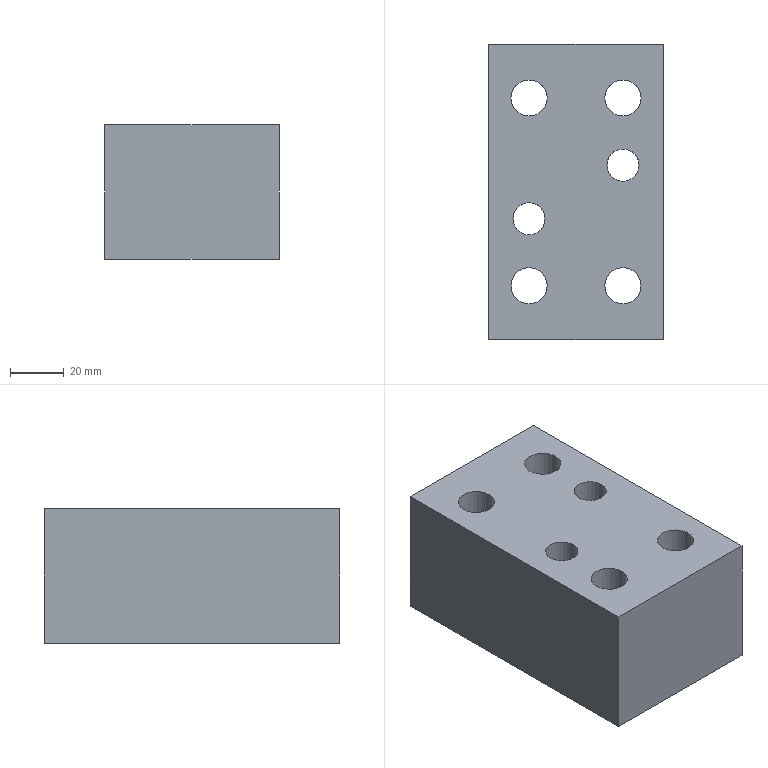Part | NX | features solid 2 | 1 solid | 20 faces | box 65 x 110 x 50 mm | volume 298901 mm3 | plane 10 | cylinder 10 | commonest cylinder face diameters 13.5 x4 19.5 x4 12 x2
STEP:
#1=CARTESIAN_POINT('',(-997.,18.,20.));
#2=VERTEX_POINT('',#1);
#3=CARTESIAN_POINT('',(-1003.,18.,20.));
#4=DIRECTION('',(0.,0.,1.));
#5=DIRECTION('',(1.,0.,0.));
#6=AXIS2_PLACEMENT_3D('',#3,#4,#5);
#7=CIRCLE('',#6,6.);
#8=EDGE_CURVE('',#2,#2,#7,.F.);
#9=ORIENTED_EDGE('',*,*,#8,.F.);
#10=EDGE_LOOP('',(#9));
#11=FACE_BOUND('',#10,.T.);
#12=CARTESIAN_POINT('',(-993.25,43.,20.));
#13=VERTEX_POINT('',#12);
#14=CARTESIAN_POINT('',(-1003.,43.,20.));
#15=DIRECTION('',(0.,0.,1.));
#16=DIRECTION('',(1.,0.,0.));
#17=AXIS2_PLACEMENT_3D('',#14,#15,#16);
#18=CIRCLE('',#17,9.75);
#19=EDGE_CURVE('',#13,#13,#18,.F.);
#20=ORIENTED_EDGE('',*,*,#19,.F.);
#21=EDGE_LOOP('',(#20));
#22=FACE_BOUND('',#21,.T.);
#23=CARTESIAN_POINT('',(-1028.25,-27.,20.));
#24=VERTEX_POINT('',#23);
#25=CARTESIAN_POINT('',(-1038.,-27.,20.));
#26=DIRECTION('',(0.,0.,1.));
#27=DIRECTION('',(1.,0.,0.));
#28=AXIS2_PLACEMENT_3D('',#25,#26,#27);
#29=CIRCLE('',#28,9.75);
#30=EDGE_CURVE('',#24,#24,#29,.F.);
#31=ORIENTED_EDGE('',*,*,#30,.F.);
#32=EDGE_LOOP('',(#31));
#33=FACE_BOUND('',#32,.T.);
#34=CARTESIAN_POINT('',(-1053.,63.,20.));
#35=VERTEX_POINT('',#34);
#36=CARTESIAN_POINT('',(-988.,63.,20.));
#37=VERTEX_POINT('',#36);
#38=CARTESIAN_POINT('',(-1028.,63.,20.));
#39=DIRECTION('',(1.,0.,0.));
#40=VECTOR('',#39,1000.);
#41=LINE('',#38,#40);
#42=EDGE_CURVE('',#35,#37,#41,.T.);
#43=ORIENTED_EDGE('',*,*,#42,.T.);
#44=CARTESIAN_POINT('',(-988.,-47.,20.));
#45=VERTEX_POINT('',#44);
#46=CARTESIAN_POINT('',(-988.,8.,20.));
#47=DIRECTION('',(0.,-1.,0.));
#48=VECTOR('',#47,1000.);
#49=LINE('',#46,#48);
#50=EDGE_CURVE('',#37,#45,#49,.T.);
#51=ORIENTED_EDGE('',*,*,#50,.T.);
#52=CARTESIAN_POINT('',(-1053.,-47.,20.));
#53=VERTEX_POINT('',#52);
#54=CARTESIAN_POINT('',(-1028.,-47.,20.));
#55=DIRECTION('',(1.,0.,0.));
#56=VECTOR('',#55,1000.);
#57=LINE('',#54,#56);
#58=EDGE_CURVE('',#53,#45,#57,.T.);
#59=ORIENTED_EDGE('',*,*,#58,.F.);
#60=CARTESIAN_POINT('',(-1053.,8.,20.));
#61=DIRECTION('',(0.,-1.,0.));
#62=VECTOR('',#61,1000.);
#63=LINE('',#60,#62);
#64=EDGE_CURVE('',#35,#53,#63,.T.);
#65=ORIENTED_EDGE('',*,*,#64,.F.);
#66=EDGE_LOOP('',(#43,#51,#59,#65));
#67=FACE_BOUND('',#66,.T.);
#68=CARTESIAN_POINT('',(-1028.25,43.,20.));
#69=VERTEX_POINT('',#68);
#70=CARTESIAN_POINT('',(-1038.,43.,20.));
#71=DIRECTION('',(0.,0.,1.));
#72=DIRECTION('',(1.,0.,0.));
#73=AXIS2_PLACEMENT_3D('',#70,#71,#72);
#74=CIRCLE('',#73,9.75);
#75=EDGE_CURVE('',#69,#69,#74,.F.);
#76=ORIENTED_EDGE('',*,*,#75,.F.);
#77=EDGE_LOOP('',(#76));
#78=FACE_BOUND('',#77,.T.);
#79=CARTESIAN_POINT('',(-993.25,-27.,20.));
#80=VERTEX_POINT('',#79);
#81=CARTESIAN_POINT('',(-1003.,-27.,20.));
#82=DIRECTION('',(0.,0.,1.));
#83=DIRECTION('',(1.,0.,0.));
#84=AXIS2_PLACEMENT_3D('',#81,#82,#83);
#85=CIRCLE('',#84,9.75);
#86=EDGE_CURVE('',#80,#80,#85,.F.);
#87=ORIENTED_EDGE('',*,*,#86,.F.);
#88=EDGE_LOOP('',(#87));
#89=FACE_BOUND('',#88,.T.);
#90=CARTESIAN_POINT('',(-1032.,-2.,20.));
#91=VERTEX_POINT('',#90);
#92=CARTESIAN_POINT('',(-1038.,-2.,20.));
#93=DIRECTION('',(0.,0.,1.));
#94=DIRECTION('',(1.,0.,0.));
#95=AXIS2_PLACEMENT_3D('',#92,#93,#94);
#96=CIRCLE('',#95,6.);
#97=EDGE_CURVE('',#91,#91,#96,.F.);
#98=ORIENTED_EDGE('',*,*,#97,.F.);
#99=EDGE_LOOP('',(#98));
#100=FACE_BOUND('',#99,.T.);
#101=CARTESIAN_POINT('',(-1028.,8.,20.));
#102=DIRECTION('',(0.,0.,1.));
#103=DIRECTION('',(0.,-1.,0.));
#104=AXIS2_PLACEMENT_3D('',#101,#102,#103);
#105=PLANE('',#104);
#106=ADVANCED_FACE('',(#11,#22,#33,#67,#78,#89,#100),#105,.F.);
#107=CARTESIAN_POINT('',(-997.,18.,70.));
#108=VERTEX_POINT('',#107);
#109=CARTESIAN_POINT('',(-1003.,18.,70.));
#110=DIRECTION('',(0.,0.,1.));
#111=DIRECTION('',(1.,0.,0.));
#112=AXIS2_PLACEMENT_3D('',#109,#110,#111);
#113=CIRCLE('',#112,6.);
#114=EDGE_CURVE('',#108,#108,#113,.F.);
#115=ORIENTED_EDGE('',*,*,#114,.T.);
#116=EDGE_LOOP('',(#115));
#117=FACE_BOUND('',#116,.T.);
#118=CARTESIAN_POINT('',(-1031.25,43.,70.));
#119=VERTEX_POINT('',#118);
#120=CARTESIAN_POINT('',(-1038.,43.,70.));
#121=DIRECTION('',(0.,0.,1.));
#122=DIRECTION('',(1.,0.,0.));
#123=AXIS2_PLACEMENT_3D('',#120,#121,#122);
#124=CIRCLE('',#123,6.75);
#125=EDGE_CURVE('',#119,#119,#124,.T.);
#126=ORIENTED_EDGE('',*,*,#125,.F.);
#127=EDGE_LOOP('',(#126));
#128=FACE_BOUND('',#127,.T.);
#129=CARTESIAN_POINT('',(-996.25,-27.,70.));
#130=VERTEX_POINT('',#129);
#131=CARTESIAN_POINT('',(-1003.,-27.,70.));
#132=DIRECTION('',(0.,0.,1.));
#133=DIRECTION('',(1.,0.,0.));
#134=AXIS2_PLACEMENT_3D('',#131,#132,#133);
#135=CIRCLE('',#134,6.75);
#136=EDGE_CURVE('',#130,#130,#135,.T.);
#137=ORIENTED_EDGE('',*,*,#136,.F.);
#138=EDGE_LOOP('',(#137));
#139=FACE_BOUND('',#138,.T.);
#140=CARTESIAN_POINT('',(-1053.,63.,70.));
#141=VERTEX_POINT('',#140);
#142=CARTESIAN_POINT('',(-988.,63.,70.));
#143=VERTEX_POINT('',#142);
#144=CARTESIAN_POINT('',(-1028.,63.,70.));
#145=DIRECTION('',(1.,0.,0.));
#146=VECTOR('',#145,1000.);
#147=LINE('',#144,#146);
#148=EDGE_CURVE('',#141,#143,#147,.T.);
#149=ORIENTED_EDGE('',*,*,#148,.F.);
#150=CARTESIAN_POINT('',(-1053.,-47.,70.));
#151=VERTEX_POINT('',#150);
#152=CARTESIAN_POINT('',(-1053.,8.,70.));
#153=DIRECTION('',(0.,-1.,0.));
#154=VECTOR('',#153,1000.);
#155=LINE('',#152,#154);
#156=EDGE_CURVE('',#141,#151,#155,.T.);
#157=ORIENTED_EDGE('',*,*,#156,.T.);
#158=CARTESIAN_POINT('',(-988.,-47.,70.));
#159=VERTEX_POINT('',#158);
#160=CARTESIAN_POINT('',(-1028.,-47.,70.));
#161=DIRECTION('',(1.,0.,0.));
#162=VECTOR('',#161,1000.);
#163=LINE('',#160,#162);
#164=EDGE_CURVE('',#151,#159,#163,.T.);
#165=ORIENTED_EDGE('',*,*,#164,.T.);
#166=CARTESIAN_POINT('',(-988.,8.,70.));
#167=DIRECTION('',(0.,-1.,0.));
#168=VECTOR('',#167,1000.);
#169=LINE('',#166,#168);
#170=EDGE_CURVE('',#143,#159,#169,.T.);
#171=ORIENTED_EDGE('',*,*,#170,.F.);
#172=EDGE_LOOP('',(#149,#157,#165,#171));
#173=FACE_BOUND('',#172,.T.);
#174=CARTESIAN_POINT('',(-1031.25,-27.,70.));
#175=VERTEX_POINT('',#174);
#176=CARTESIAN_POINT('',(-1038.,-27.,70.));
#177=DIRECTION('',(0.,0.,1.));
#178=DIRECTION('',(1.,0.,0.));
#179=AXIS2_PLACEMENT_3D('',#176,#177,#178);
#180=CIRCLE('',#179,6.75);
#181=EDGE_CURVE('',#175,#175,#180,.T.);
#182=ORIENTED_EDGE('',*,*,#181,.F.);
#183=EDGE_LOOP('',(#182));
#184=FACE_BOUND('',#183,.T.);
#185=CARTESIAN_POINT('',(-996.25,43.,70.));
#186=VERTEX_POINT('',#185);
#187=CARTESIAN_POINT('',(-1003.,43.,70.));
#188=DIRECTION('',(0.,0.,1.));
#189=DIRECTION('',(1.,0.,0.));
#190=AXIS2_PLACEMENT_3D('',#187,#188,#189);
#191=CIRCLE('',#190,6.75);
#192=EDGE_CURVE('',#186,#186,#191,.T.);
#193=ORIENTED_EDGE('',*,*,#192,.F.);
#194=EDGE_LOOP('',(#193));
#195=FACE_BOUND('',#194,.T.);
#196=CARTESIAN_POINT('',(-1032.,-2.,70.));
#197=VERTEX_POINT('',#196);
#198=CARTESIAN_POINT('',(-1038.,-2.,70.));
#199=DIRECTION('',(0.,0.,1.));
#200=DIRECTION('',(1.,0.,0.));
#201=AXIS2_PLACEMENT_3D('',#198,#199,#200);
#202=CIRCLE('',#201,6.);
#203=EDGE_CURVE('',#197,#197,#202,.F.);
#204=ORIENTED_EDGE('',*,*,#203,.T.);
#205=EDGE_LOOP('',(#204));
#206=FACE_BOUND('',#205,.T.);
#207=CARTESIAN_POINT('',(-1028.,8.,70.));
#208=DIRECTION('',(0.,0.,1.));
#209=DIRECTION('',(0.,-1.,0.));
#210=AXIS2_PLACEMENT_3D('',#207,#208,#209);
#211=PLANE('',#210);
#212=ADVANCED_FACE('',(#117,#128,#139,#173,#184,#195,#206),#211,.T.);
#213=ORIENTED_EDGE('',*,*,#42,.F.);
#214=CARTESIAN_POINT('',(-1053.,63.,220.));
#215=DIRECTION('',(0.,0.,-1.));
#216=VECTOR('',#215,1000.);
#217=LINE('',#214,#216);
#218=EDGE_CURVE('',#141,#35,#217,.T.);
#219=ORIENTED_EDGE('',*,*,#218,.F.);
#220=ORIENTED_EDGE('',*,*,#148,.T.);
#221=CARTESIAN_POINT('',(-988.,63.,220.));
#222=DIRECTION('',(0.,0.,-1.));
#223=VECTOR('',#222,1000.);
#224=LINE('',#221,#223);
#225=EDGE_CURVE('',#143,#37,#224,.T.);
#226=ORIENTED_EDGE('',*,*,#225,.T.);
#227=EDGE_LOOP('',(#213,#219,#220,#226));
#228=FACE_BOUND('',#227,.T.);
#229=CARTESIAN_POINT('',(-1028.,63.,220.));
#230=DIRECTION('',(0.,1.,0.));
#231=DIRECTION('',(0.,0.,1.));
#232=AXIS2_PLACEMENT_3D('',#229,#230,#231);
#233=PLANE('',#232);
#234=ADVANCED_FACE('',(#228),#233,.T.);
#235=ORIENTED_EDGE('',*,*,#64,.T.);
#236=CARTESIAN_POINT('',(-1053.,-47.,220.));
#237=DIRECTION('',(0.,0.,-1.));
#238=VECTOR('',#237,1000.);
#239=LINE('',#236,#238);
#240=EDGE_CURVE('',#151,#53,#239,.T.);
#241=ORIENTED_EDGE('',*,*,#240,.F.);
#242=ORIENTED_EDGE('',*,*,#156,.F.);
#243=ORIENTED_EDGE('',*,*,#218,.T.);
#244=EDGE_LOOP('',(#235,#241,#242,#243));
#245=FACE_BOUND('',#244,.T.);
#246=CARTESIAN_POINT('',(-1053.,8.,220.));
#247=DIRECTION('',(1.,0.,0.));
#248=DIRECTION('',(0.,0.,-1.));
#249=AXIS2_PLACEMENT_3D('',#246,#247,#248);
#250=PLANE('',#249);
#251=ADVANCED_FACE('',(#245),#250,.F.);
#252=ORIENTED_EDGE('',*,*,#58,.T.);
#253=CARTESIAN_POINT('',(-988.,-47.,220.));
#254=DIRECTION('',(0.,0.,-1.));
#255=VECTOR('',#254,1000.);
#256=LINE('',#253,#255);
#257=EDGE_CURVE('',#159,#45,#256,.T.);
#258=ORIENTED_EDGE('',*,*,#257,.F.);
#259=ORIENTED_EDGE('',*,*,#164,.F.);
#260=ORIENTED_EDGE('',*,*,#240,.T.);
#261=EDGE_LOOP('',(#252,#258,#259,#260));
#262=FACE_BOUND('',#261,.T.);
#263=CARTESIAN_POINT('',(-1028.,-47.,220.));
#264=DIRECTION('',(0.,1.,0.));
#265=DIRECTION('',(0.,0.,1.));
#266=AXIS2_PLACEMENT_3D('',#263,#264,#265);
#267=PLANE('',#266);
#268=ADVANCED_FACE('',(#262),#267,.F.);
#269=ORIENTED_EDGE('',*,*,#50,.F.);
#270=ORIENTED_EDGE('',*,*,#225,.F.);
#271=ORIENTED_EDGE('',*,*,#170,.T.);
#272=ORIENTED_EDGE('',*,*,#257,.T.);
#273=EDGE_LOOP('',(#269,#270,#271,#272));
#274=FACE_BOUND('',#273,.T.);
#275=CARTESIAN_POINT('',(-988.,8.,220.));
#276=DIRECTION('',(1.,0.,0.));
#277=DIRECTION('',(0.,0.,-1.));
#278=AXIS2_PLACEMENT_3D('',#275,#276,#277);
#279=PLANE('',#278);
#280=ADVANCED_FACE('',(#274),#279,.T.);
#281=CARTESIAN_POINT('',(-996.25,-27.,50.));
#282=VERTEX_POINT('',#281);
#283=CARTESIAN_POINT('',(-1003.,-27.,50.));
#284=DIRECTION('',(0.,0.,1.));
#285=DIRECTION('',(1.,0.,0.));
#286=AXIS2_PLACEMENT_3D('',#283,#284,#285);
#287=CIRCLE('',#286,6.75);
#288=EDGE_CURVE('',#282,#282,#287,.T.);
#289=ORIENTED_EDGE('',*,*,#288,.F.);
#290=EDGE_LOOP('',(#289));
#291=FACE_BOUND('',#290,.T.);
#292=ORIENTED_EDGE('',*,*,#136,.T.);
#293=EDGE_LOOP('',(#292));
#294=FACE_BOUND('',#293,.T.);
#295=CARTESIAN_POINT('',(-1003.,-27.,70.));
#296=DIRECTION('',(0.,0.,-1.));
#297=DIRECTION('',(-1.,0.,0.));
#298=AXIS2_PLACEMENT_3D('',#295,#296,#297);
#299=CYLINDRICAL_SURFACE('',#298,6.75);
#300=ADVANCED_FACE('',(#291,#294),#299,.F.);
#301=CARTESIAN_POINT('',(-1031.25,-27.,50.));
#302=VERTEX_POINT('',#301);
#303=CARTESIAN_POINT('',(-1038.,-27.,50.));
#304=DIRECTION('',(0.,0.,1.));
#305=DIRECTION('',(1.,0.,0.));
#306=AXIS2_PLACEMENT_3D('',#303,#304,#305);
#307=CIRCLE('',#306,6.75);
#308=EDGE_CURVE('',#302,#302,#307,.T.);
#309=ORIENTED_EDGE('',*,*,#308,.F.);
#310=EDGE_LOOP('',(#309));
#311=FACE_BOUND('',#310,.T.);
#312=ORIENTED_EDGE('',*,*,#181,.T.);
#313=EDGE_LOOP('',(#312));
#314=FACE_BOUND('',#313,.T.);
#315=CARTESIAN_POINT('',(-1038.,-27.,70.));
#316=DIRECTION('',(0.,0.,-1.));
#317=DIRECTION('',(-1.,0.,0.));
#318=AXIS2_PLACEMENT_3D('',#315,#316,#317);
#319=CYLINDRICAL_SURFACE('',#318,6.75);
#320=ADVANCED_FACE('',(#311,#314),#319,.F.);
#321=CARTESIAN_POINT('',(-1031.25,43.,50.));
#322=VERTEX_POINT('',#321);
#323=CARTESIAN_POINT('',(-1038.,43.,50.));
#324=DIRECTION('',(0.,0.,1.));
#325=DIRECTION('',(1.,0.,0.));
#326=AXIS2_PLACEMENT_3D('',#323,#324,#325);
#327=CIRCLE('',#326,6.75);
#328=EDGE_CURVE('',#322,#322,#327,.T.);
#329=ORIENTED_EDGE('',*,*,#328,.F.);
#330=EDGE_LOOP('',(#329));
#331=FACE_BOUND('',#330,.T.);
#332=ORIENTED_EDGE('',*,*,#125,.T.);
#333=EDGE_LOOP('',(#332));
#334=FACE_BOUND('',#333,.T.);
#335=CARTESIAN_POINT('',(-1038.,43.,70.));
#336=DIRECTION('',(0.,0.,-1.));
#337=DIRECTION('',(-1.,0.,0.));
#338=AXIS2_PLACEMENT_3D('',#335,#336,#337);
#339=CYLINDRICAL_SURFACE('',#338,6.75);
#340=ADVANCED_FACE('',(#331,#334),#339,.F.);
#341=CARTESIAN_POINT('',(-996.25,43.,50.));
#342=VERTEX_POINT('',#341);
#343=CARTESIAN_POINT('',(-1003.,43.,50.));
#344=DIRECTION('',(0.,0.,1.));
#345=DIRECTION('',(1.,0.,0.));
#346=AXIS2_PLACEMENT_3D('',#343,#344,#345);
#347=CIRCLE('',#346,6.75);
#348=EDGE_CURVE('',#342,#342,#347,.T.);
#349=ORIENTED_EDGE('',*,*,#348,.F.);
#350=EDGE_LOOP('',(#349));
#351=FACE_BOUND('',#350,.T.);
#352=ORIENTED_EDGE('',*,*,#192,.T.);
#353=EDGE_LOOP('',(#352));
#354=FACE_BOUND('',#353,.T.);
#355=CARTESIAN_POINT('',(-1003.,43.,70.));
#356=DIRECTION('',(0.,0.,-1.));
#357=DIRECTION('',(-1.,0.,0.));
#358=AXIS2_PLACEMENT_3D('',#355,#356,#357);
#359=CYLINDRICAL_SURFACE('',#358,6.75);
#360=ADVANCED_FACE('',(#351,#354),#359,.F.);
#361=CARTESIAN_POINT('',(-1028.25,-27.,50.));
#362=VERTEX_POINT('',#361);
#363=CARTESIAN_POINT('',(-1038.,-27.,50.));
#364=DIRECTION('',(0.,0.,1.));
#365=DIRECTION('',(1.,0.,0.));
#366=AXIS2_PLACEMENT_3D('',#363,#364,#365);
#367=CIRCLE('',#366,9.75);
#368=EDGE_CURVE('',#362,#362,#367,.T.);
#369=ORIENTED_EDGE('',*,*,#368,.T.);
#370=EDGE_LOOP('',(#369));
#371=FACE_BOUND('',#370,.T.);
#372=ORIENTED_EDGE('',*,*,#30,.T.);
#373=EDGE_LOOP('',(#372));
#374=FACE_BOUND('',#373,.T.);
#375=CARTESIAN_POINT('',(-1038.,-27.,50.));
#376=DIRECTION('',(0.,0.,-1.));
#377=DIRECTION('',(-1.,0.,0.));
#378=AXIS2_PLACEMENT_3D('',#375,#376,#377);
#379=CYLINDRICAL_SURFACE('',#378,9.75);
#380=ADVANCED_FACE('',(#371,#374),#379,.F.);
#381=ORIENTED_EDGE('',*,*,#308,.T.);
#382=EDGE_LOOP('',(#381));
#383=FACE_BOUND('',#382,.T.);
#384=ORIENTED_EDGE('',*,*,#368,.F.);
#385=EDGE_LOOP('',(#384));
#386=FACE_BOUND('',#385,.T.);
#387=CARTESIAN_POINT('',(-1038.,-32.,50.));
#388=DIRECTION('',(0.,0.,1.));
#389=DIRECTION('',(1.,0.,0.));
#390=AXIS2_PLACEMENT_3D('',#387,#388,#389);
#391=PLANE('',#390);
#392=ADVANCED_FACE('',(#383,#386),#391,.F.);
#393=CARTESIAN_POINT('',(-1028.25,43.,50.));
#394=VERTEX_POINT('',#393);
#395=CARTESIAN_POINT('',(-1038.,43.,50.));
#396=DIRECTION('',(0.,0.,1.));
#397=DIRECTION('',(1.,0.,0.));
#398=AXIS2_PLACEMENT_3D('',#395,#396,#397);
#399=CIRCLE('',#398,9.75);
#400=EDGE_CURVE('',#394,#394,#399,.T.);
#401=ORIENTED_EDGE('',*,*,#400,.T.);
#402=EDGE_LOOP('',(#401));
#403=FACE_BOUND('',#402,.T.);
#404=ORIENTED_EDGE('',*,*,#75,.T.);
#405=EDGE_LOOP('',(#404));
#406=FACE_BOUND('',#405,.T.);
#407=CARTESIAN_POINT('',(-1038.,43.,50.));
#408=DIRECTION('',(0.,0.,-1.));
#409=DIRECTION('',(-1.,0.,0.));
#410=AXIS2_PLACEMENT_3D('',#407,#408,#409);
#411=CYLINDRICAL_SURFACE('',#410,9.75);
#412=ADVANCED_FACE('',(#403,#406),#411,.F.);
#413=ORIENTED_EDGE('',*,*,#328,.T.);
#414=EDGE_LOOP('',(#413));
#415=FACE_BOUND('',#414,.T.);
#416=ORIENTED_EDGE('',*,*,#400,.F.);
#417=EDGE_LOOP('',(#416));
#418=FACE_BOUND('',#417,.T.);
#419=CARTESIAN_POINT('',(-1038.,48.,50.));
#420=DIRECTION('',(0.,0.,1.));
#421=DIRECTION('',(1.,0.,0.));
#422=AXIS2_PLACEMENT_3D('',#419,#420,#421);
#423=PLANE('',#422);
#424=ADVANCED_FACE('',(#415,#418),#423,.F.);
#425=CARTESIAN_POINT('',(-993.25,43.,50.));
#426=VERTEX_POINT('',#425);
#427=CARTESIAN_POINT('',(-1003.,43.,50.));
#428=DIRECTION('',(0.,0.,1.));
#429=DIRECTION('',(1.,0.,0.));
#430=AXIS2_PLACEMENT_3D('',#427,#428,#429);
#431=CIRCLE('',#430,9.75);
#432=EDGE_CURVE('',#426,#426,#431,.T.);
#433=ORIENTED_EDGE('',*,*,#432,.T.);
#434=EDGE_LOOP('',(#433));
#435=FACE_BOUND('',#434,.T.);
#436=ORIENTED_EDGE('',*,*,#19,.T.);
#437=EDGE_LOOP('',(#436));
#438=FACE_BOUND('',#437,.T.);
#439=CARTESIAN_POINT('',(-1003.,43.,50.));
#440=DIRECTION('',(0.,0.,-1.));
#441=DIRECTION('',(-1.,0.,0.));
#442=AXIS2_PLACEMENT_3D('',#439,#440,#441);
#443=CYLINDRICAL_SURFACE('',#442,9.75);
#444=ADVANCED_FACE('',(#435,#438),#443,.F.);
#445=ORIENTED_EDGE('',*,*,#348,.T.);
#446=EDGE_LOOP('',(#445));
#447=FACE_BOUND('',#446,.T.);
#448=ORIENTED_EDGE('',*,*,#432,.F.);
#449=EDGE_LOOP('',(#448));
#450=FACE_BOUND('',#449,.T.);
#451=CARTESIAN_POINT('',(-1003.,48.,50.));
#452=DIRECTION('',(0.,0.,1.));
#453=DIRECTION('',(1.,0.,0.));
#454=AXIS2_PLACEMENT_3D('',#451,#452,#453);
#455=PLANE('',#454);
#456=ADVANCED_FACE('',(#447,#450),#455,.F.);
#457=CARTESIAN_POINT('',(-993.25,-27.,50.));
#458=VERTEX_POINT('',#457);
#459=CARTESIAN_POINT('',(-1003.,-27.,50.));
#460=DIRECTION('',(0.,0.,1.));
#461=DIRECTION('',(1.,0.,0.));
#462=AXIS2_PLACEMENT_3D('',#459,#460,#461);
#463=CIRCLE('',#462,9.75);
#464=EDGE_CURVE('',#458,#458,#463,.T.);
#465=ORIENTED_EDGE('',*,*,#464,.T.);
#466=EDGE_LOOP('',(#465));
#467=FACE_BOUND('',#466,.T.);
#468=ORIENTED_EDGE('',*,*,#86,.T.);
#469=EDGE_LOOP('',(#468));
#470=FACE_BOUND('',#469,.T.);
#471=CARTESIAN_POINT('',(-1003.,-27.,50.));
#472=DIRECTION('',(0.,0.,-1.));
#473=DIRECTION('',(-1.,0.,0.));
#474=AXIS2_PLACEMENT_3D('',#471,#472,#473);
#475=CYLINDRICAL_SURFACE('',#474,9.75);
#476=ADVANCED_FACE('',(#467,#470),#475,.F.);
#477=ORIENTED_EDGE('',*,*,#288,.T.);
#478=EDGE_LOOP('',(#477));
#479=FACE_BOUND('',#478,.T.);
#480=ORIENTED_EDGE('',*,*,#464,.F.);
#481=EDGE_LOOP('',(#480));
#482=FACE_BOUND('',#481,.T.);
#483=CARTESIAN_POINT('',(-1003.,-32.,50.));
#484=DIRECTION('',(0.,0.,1.));
#485=DIRECTION('',(1.,0.,0.));
#486=AXIS2_PLACEMENT_3D('',#483,#484,#485);
#487=PLANE('',#486);
#488=ADVANCED_FACE('',(#479,#482),#487,.F.);
#489=ORIENTED_EDGE('',*,*,#114,.F.);
#490=EDGE_LOOP('',(#489));
#491=FACE_BOUND('',#490,.T.);
#492=ORIENTED_EDGE('',*,*,#8,.T.);
#493=EDGE_LOOP('',(#492));
#494=FACE_BOUND('',#493,.T.);
#495=CARTESIAN_POINT('',(-1003.,18.,550.));
#496=DIRECTION('',(0.,0.,-1.));
#497=DIRECTION('',(-1.,0.,0.));
#498=AXIS2_PLACEMENT_3D('',#495,#496,#497);
#499=CYLINDRICAL_SURFACE('',#498,6.);
#500=ADVANCED_FACE('',(#491,#494),#499,.F.);
#501=ORIENTED_EDGE('',*,*,#203,.F.);
#502=EDGE_LOOP('',(#501));
#503=FACE_BOUND('',#502,.T.);
#504=ORIENTED_EDGE('',*,*,#97,.T.);
#505=EDGE_LOOP('',(#504));
#506=FACE_BOUND('',#505,.T.);
#507=CARTESIAN_POINT('',(-1038.,-2.,550.));
#508=DIRECTION('',(0.,0.,-1.));
#509=DIRECTION('',(-1.,0.,0.));
#510=AXIS2_PLACEMENT_3D('',#507,#508,#509);
#511=CYLINDRICAL_SURFACE('',#510,6.);
#512=ADVANCED_FACE('',(#503,#506),#511,.F.);
#513=CLOSED_SHELL('',(#106,#212,#234,#251,#268,#280,#300,#320,#340,#360,#380,#392,#412,#424,#444,#456,#476,#488,#500,#512));
#514=MANIFOLD_SOLID_BREP('',#513);
#515=(LENGTH_UNIT()NAMED_UNIT(*)SI_UNIT(.MILLI.,.METRE.));
#516=UNCERTAINTY_MEASURE_WITH_UNIT(LENGTH_MEASURE(0.00001),#515,'','');
#517=(NAMED_UNIT(*)PLANE_ANGLE_UNIT()SI_UNIT($,.RADIAN.));
#518=(NAMED_UNIT(*)SI_UNIT($,.STERADIAN.)SOLID_ANGLE_UNIT());
#519=(GEOMETRIC_REPRESENTATION_CONTEXT(3)GLOBAL_UNCERTAINTY_ASSIGNED_CONTEXT((#516))GLOBAL_UNIT_ASSIGNED_CONTEXT((#515,#517,#518))REPRESENTATION_CONTEXT('',''));
#520=ADVANCED_BREP_SHAPE_REPRESENTATION('',(#514),#519);